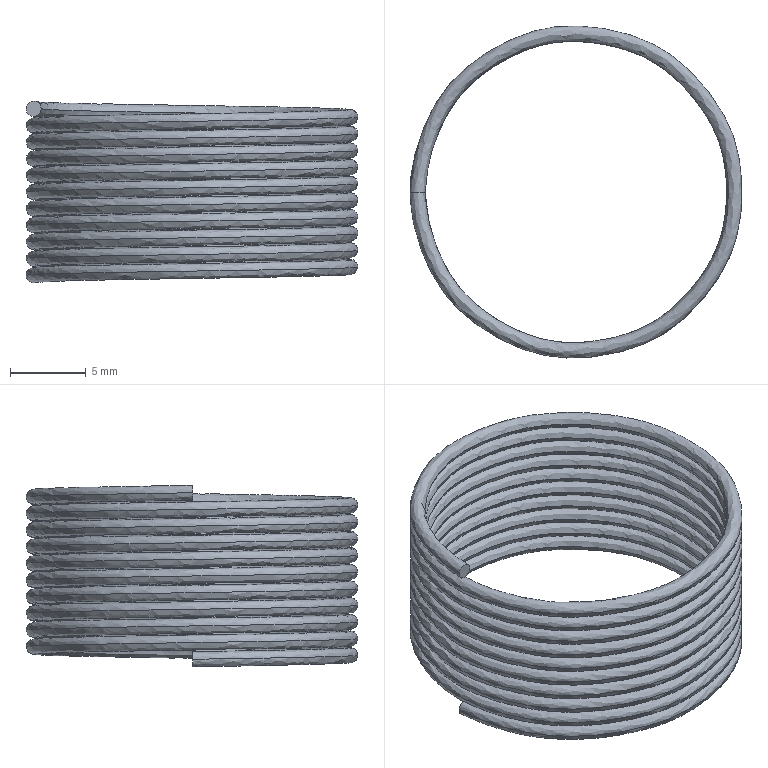Part | SolidWorks | features BaseBody 1 | 1 solid | 4 faces | box 21.937 x 21.934 x 11.998 mm | volume 512.646 mm3 | spline 2 | plane 2